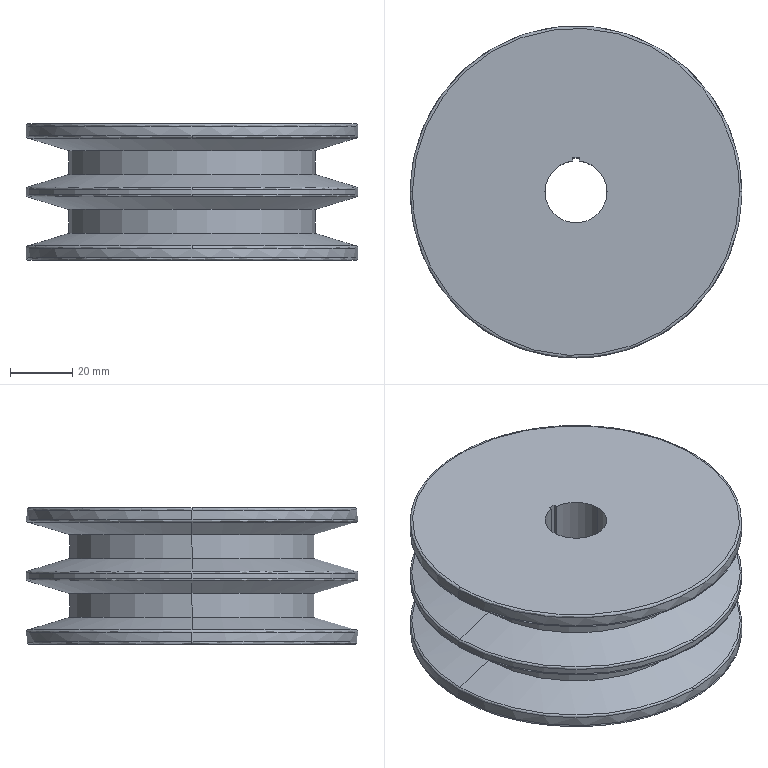Part | SolidWorks | features ICE 3, BaseBody 1 | 1 solid | 38 faces | box 107 x 107 x 44 mm | volume 283777 mm3 | cylinder 13 | spline 12 | cone 8 | plane 5 | commonest cylinder face diameters 107 x6 79.502 x4 20 x3
STEP:
#1=CARTESIAN_POINT('',(-52.969,0.,-4.592));
#2=VERTEX_POINT('',#1);
#3=CARTESIAN_POINT('',(0.,-52.969,-4.592));
#4=VERTEX_POINT('',#3);
#5=CARTESIAN_POINT('',(0.,0.,-4.592));
#6=DIRECTION('',(0.,0.,1.));
#7=DIRECTION('',(0.,1.,0.));
#8=AXIS2_PLACEMENT_3D('',#5,#6,#7);
#9=CIRCLE('',#8,52.969);
#10=EDGE_CURVE('',#2,#4,#9,.T.);
#11=ORIENTED_EDGE('',*,*,#10,.T.);
#12=CARTESIAN_POINT('',(0.,-53.5,-3.875));
#13=VERTEX_POINT('',#12);
#14=CARTESIAN_POINT('',(0.,-52.75,-3.875));
#15=DIRECTION('',(-1.,0.,0.));
#16=DIRECTION('',(0.,-1.,0.));
#17=AXIS2_PLACEMENT_3D('',#14,#15,#16);
#18=CIRCLE('',#17,0.75);
#19=EDGE_CURVE('',#4,#13,#18,.T.);
#20=ORIENTED_EDGE('',*,*,#19,.T.);
#21=CARTESIAN_POINT('',(-53.5,0.,-3.875));
#22=VERTEX_POINT('',#21);
#23=CARTESIAN_POINT('',(0.,0.,-3.875));
#24=DIRECTION('',(0.,0.,1.));
#25=DIRECTION('',(1.,0.,0.));
#26=AXIS2_PLACEMENT_3D('',#23,#24,#25);
#27=CIRCLE('',#26,53.5);
#28=EDGE_CURVE('',#22,#13,#27,.T.);
#29=ORIENTED_EDGE('',*,*,#28,.F.);
#30=CARTESIAN_POINT('',(0.,53.5,-3.875));
#31=VERTEX_POINT('',#30);
#32=CARTESIAN_POINT('',(0.,0.,-3.875));
#33=DIRECTION('',(0.,0.,1.));
#34=DIRECTION('',(1.,0.,0.));
#35=AXIS2_PLACEMENT_3D('',#32,#33,#34);
#36=CIRCLE('',#35,53.5);
#37=EDGE_CURVE('',#31,#22,#36,.T.);
#38=ORIENTED_EDGE('',*,*,#37,.F.);
#39=CARTESIAN_POINT('',(0.,52.969,-4.592));
#40=VERTEX_POINT('',#39);
#41=CARTESIAN_POINT('',(0.,52.75,-3.875));
#42=DIRECTION('',(1.,0.,0.));
#43=DIRECTION('',(0.,1.,0.));
#44=AXIS2_PLACEMENT_3D('',#41,#42,#43);
#45=CIRCLE('',#44,0.75);
#46=EDGE_CURVE('',#40,#31,#45,.T.);
#47=ORIENTED_EDGE('',*,*,#46,.F.);
#48=CARTESIAN_POINT('',(0.,0.,-4.592));
#49=DIRECTION('',(0.,0.,1.));
#50=DIRECTION('',(0.,1.,0.));
#51=AXIS2_PLACEMENT_3D('',#48,#49,#50);
#52=CIRCLE('',#51,52.969);
#53=EDGE_CURVE('',#40,#2,#52,.T.);
#54=ORIENTED_EDGE('',*,*,#53,.T.);
#55=EDGE_LOOP('',(#11,#20,#29,#38,#47,#54));
#56=FACE_OUTER_BOUND('',#55,.T.);
#57=CARTESIAN_POINT('',(0.,-52.969,-4.592));
#58=CARTESIAN_POINT('',(-105.939,-52.969,-4.592));
#59=CARTESIAN_POINT('',(-105.939,52.969,-4.592));
#60=CARTESIAN_POINT('',(0.,52.969,-4.592));
#61=CARTESIAN_POINT('',(0.,-53.296,-4.492));
#62=CARTESIAN_POINT('',(-106.593,-53.296,-4.492));
#63=CARTESIAN_POINT('',(-106.593,53.296,-4.492));
#64=CARTESIAN_POINT('',(0.,53.296,-4.492));
#65=CARTESIAN_POINT('',(0.,-53.5,-4.217));
#66=CARTESIAN_POINT('',(-107.,-53.5,-4.217));
#67=CARTESIAN_POINT('',(-107.,53.5,-4.217));
#68=CARTESIAN_POINT('',(0.,53.5,-4.217));
#69=CARTESIAN_POINT('',(0.,-53.5,-3.875));
#70=CARTESIAN_POINT('',(-107.,-53.5,-3.875));
#71=CARTESIAN_POINT('',(-107.,53.5,-3.875));
#72=CARTESIAN_POINT('',(0.,53.5,-3.875));
#73=(BOUNDED_SURFACE()B_SPLINE_SURFACE(3,3,((#57,#58,#59,#60),(#61,#62,#63,#64),(#65,#66,#67,#68),(#69,#70,#71,#72)),.UNSPECIFIED.,.F.,.F.,.F.)B_SPLINE_SURFACE_WITH_KNOTS((4,4),(4,4),(0.,1.),(0.,1.),.UNSPECIFIED.)GEOMETRIC_REPRESENTATION_ITEM()RATIONAL_B_SPLINE_SURFACE(((1.,0.3333,0.3333,1.),(0.8692,0.2897,0.2897,0.8692),(0.8692,0.2897,0.2897,0.8692),(1.,0.3333,0.3333,1.)))REPRESENTATION_ITEM('')SURFACE());
#74=ADVANCED_FACE('',(#56),#73,.T.);
#75=CARTESIAN_POINT('',(-53.5,0.,-0.75));
#76=VERTEX_POINT('',#75);
#77=CARTESIAN_POINT('',(53.5,0.,-0.75));
#78=VERTEX_POINT('',#77);
#79=CARTESIAN_POINT('',(0.,0.,-0.75));
#80=DIRECTION('',(0.,0.,1.));
#81=DIRECTION('',(-1.,0.,0.));
#82=AXIS2_PLACEMENT_3D('',#79,#80,#81);
#83=CIRCLE('',#82,53.5);
#84=EDGE_CURVE('',#76,#78,#83,.T.);
#85=ORIENTED_EDGE('',*,*,#84,.T.);
#86=CARTESIAN_POINT('',(52.75,0.,0.));
#87=VERTEX_POINT('',#86);
#88=CARTESIAN_POINT('',(52.75,0.,-0.75));
#89=DIRECTION('',(0.,-1.,0.));
#90=DIRECTION('',(1.,0.,0.));
#91=AXIS2_PLACEMENT_3D('',#88,#89,#90);
#92=CIRCLE('',#91,0.75);
#93=EDGE_CURVE('',#78,#87,#92,.T.);
#94=ORIENTED_EDGE('',*,*,#93,.T.);
#95=CARTESIAN_POINT('',(-52.75,0.,0.));
#96=VERTEX_POINT('',#95);
#97=CARTESIAN_POINT('',(52.75,0.,0.));
#98=CARTESIAN_POINT('',(52.75,-105.5,0.));
#99=CARTESIAN_POINT('',(-52.75,-105.5,0.));
#100=CARTESIAN_POINT('',(-52.75,0.,0.));
#101=(BOUNDED_CURVE()B_SPLINE_CURVE(3,(#97,#98,#99,#100),.UNSPECIFIED.,.F.,.F.)B_SPLINE_CURVE_WITH_KNOTS((4,4),(0.,1.),.UNSPECIFIED.)CURVE()GEOMETRIC_REPRESENTATION_ITEM()RATIONAL_B_SPLINE_CURVE((1.,0.3333,0.3333,1.))REPRESENTATION_ITEM(''));
#102=EDGE_CURVE('',#87,#96,#101,.T.);
#103=ORIENTED_EDGE('',*,*,#102,.T.);
#104=CARTESIAN_POINT('',(-52.75,0.,-0.75));
#105=DIRECTION('',(0.,1.,0.));
#106=DIRECTION('',(-1.,0.,0.));
#107=AXIS2_PLACEMENT_3D('',#104,#105,#106);
#108=CIRCLE('',#107,0.75);
#109=EDGE_CURVE('',#76,#96,#108,.T.);
#110=ORIENTED_EDGE('',*,*,#109,.F.);
#111=EDGE_LOOP('',(#85,#94,#103,#110));
#112=FACE_OUTER_BOUND('',#111,.T.);
#113=CARTESIAN_POINT('',(53.5,0.,-0.75));
#114=CARTESIAN_POINT('',(53.5,-107.,-0.75));
#115=CARTESIAN_POINT('',(-53.5,-107.,-0.75));
#116=CARTESIAN_POINT('',(-53.5,0.,-0.75));
#117=CARTESIAN_POINT('',(53.5,0.,-0.3107));
#118=CARTESIAN_POINT('',(53.5,-107.,-0.3107));
#119=CARTESIAN_POINT('',(-53.5,-107.,-0.3107));
#120=CARTESIAN_POINT('',(-53.5,0.,-0.3107));
#121=CARTESIAN_POINT('',(53.189,0.,0.));
#122=CARTESIAN_POINT('',(53.189,-106.379,0.));
#123=CARTESIAN_POINT('',(-53.189,-106.379,0.));
#124=CARTESIAN_POINT('',(-53.189,0.,0.));
#125=CARTESIAN_POINT('',(52.75,0.,0.));
#126=CARTESIAN_POINT('',(52.75,-105.5,0.));
#127=CARTESIAN_POINT('',(-52.75,-105.5,0.));
#128=CARTESIAN_POINT('',(-52.75,0.,0.));
#129=(BOUNDED_SURFACE()B_SPLINE_SURFACE(3,3,((#113,#114,#115,#116),(#117,#118,#119,#120),(#121,#122,#123,#124),(#125,#126,#127,#128)),.UNSPECIFIED.,.F.,.F.,.T.)B_SPLINE_SURFACE_WITH_KNOTS((4,4),(4,4),(0.,1.),(0.,1.),.UNSPECIFIED.)GEOMETRIC_REPRESENTATION_ITEM()RATIONAL_B_SPLINE_SURFACE(((1.,0.3333,0.3333,1.),(0.8047,0.2682,0.2682,0.8047),(0.8047,0.2682,0.2682,0.8047),(1.,0.3333,0.3333,1.)))REPRESENTATION_ITEM('')SURFACE());
#130=ADVANCED_FACE('',(#112),#129,.T.);
#131=CARTESIAN_POINT('',(-53.5,0.,-21.125));
#132=VERTEX_POINT('',#131);
#133=CARTESIAN_POINT('',(0.,-53.5,-21.125));
#134=VERTEX_POINT('',#133);
#135=CARTESIAN_POINT('',(0.,0.,-21.125));
#136=DIRECTION('',(0.,0.,1.));
#137=DIRECTION('',(0.,1.,0.));
#138=AXIS2_PLACEMENT_3D('',#135,#136,#137);
#139=CIRCLE('',#138,53.5);
#140=EDGE_CURVE('',#132,#134,#139,.T.);
#141=ORIENTED_EDGE('',*,*,#140,.T.);
#142=CARTESIAN_POINT('',(0.,-52.969,-20.408));
#143=VERTEX_POINT('',#142);
#144=CARTESIAN_POINT('',(0.,-52.75,-21.125));
#145=DIRECTION('',(-1.,0.,0.));
#146=DIRECTION('',(0.,-1.,0.));
#147=AXIS2_PLACEMENT_3D('',#144,#145,#146);
#148=CIRCLE('',#147,0.75);
#149=EDGE_CURVE('',#134,#143,#148,.T.);
#150=ORIENTED_EDGE('',*,*,#149,.T.);
#151=CARTESIAN_POINT('',(-52.969,0.,-20.408));
#152=VERTEX_POINT('',#151);
#153=CARTESIAN_POINT('',(0.,0.,-20.408));
#154=DIRECTION('',(0.,0.,1.));
#155=DIRECTION('',(0.,1.,0.));
#156=AXIS2_PLACEMENT_3D('',#153,#154,#155);
#157=CIRCLE('',#156,52.969);
#158=EDGE_CURVE('',#152,#143,#157,.T.);
#159=ORIENTED_EDGE('',*,*,#158,.F.);
#160=CARTESIAN_POINT('',(0.,52.969,-20.408));
#161=VERTEX_POINT('',#160);
#162=CARTESIAN_POINT('',(0.,0.,-20.408));
#163=DIRECTION('',(0.,0.,1.));
#164=DIRECTION('',(0.,1.,0.));
#165=AXIS2_PLACEMENT_3D('',#162,#163,#164);
#166=CIRCLE('',#165,52.969);
#167=EDGE_CURVE('',#161,#152,#166,.T.);
#168=ORIENTED_EDGE('',*,*,#167,.F.);
#169=CARTESIAN_POINT('',(0.,53.5,-21.125));
#170=VERTEX_POINT('',#169);
#171=CARTESIAN_POINT('',(0.,52.75,-21.125));
#172=DIRECTION('',(1.,0.,0.));
#173=DIRECTION('',(0.,1.,0.));
#174=AXIS2_PLACEMENT_3D('',#171,#172,#173);
#175=CIRCLE('',#174,0.75);
#176=EDGE_CURVE('',#170,#161,#175,.T.);
#177=ORIENTED_EDGE('',*,*,#176,.F.);
#178=CARTESIAN_POINT('',(0.,0.,-21.125));
#179=DIRECTION('',(0.,0.,1.));
#180=DIRECTION('',(0.,1.,0.));
#181=AXIS2_PLACEMENT_3D('',#178,#179,#180);
#182=CIRCLE('',#181,53.5);
#183=EDGE_CURVE('',#170,#132,#182,.T.);
#184=ORIENTED_EDGE('',*,*,#183,.T.);
#185=EDGE_LOOP('',(#141,#150,#159,#168,#177,#184));
#186=FACE_OUTER_BOUND('',#185,.T.);
#187=CARTESIAN_POINT('',(0.,-53.5,-21.125));
#188=CARTESIAN_POINT('',(-107.,-53.5,-21.125));
#189=CARTESIAN_POINT('',(-107.,53.5,-21.125));
#190=CARTESIAN_POINT('',(0.,53.5,-21.125));
#191=CARTESIAN_POINT('',(0.,-53.5,-20.783));
#192=CARTESIAN_POINT('',(-107.,-53.5,-20.783));
#193=CARTESIAN_POINT('',(-107.,53.5,-20.783));
#194=CARTESIAN_POINT('',(0.,53.5,-20.783));
#195=CARTESIAN_POINT('',(0.,-53.296,-20.508));
#196=CARTESIAN_POINT('',(-106.593,-53.296,-20.508));
#197=CARTESIAN_POINT('',(-106.593,53.296,-20.508));
#198=CARTESIAN_POINT('',(0.,53.296,-20.508));
#199=CARTESIAN_POINT('',(0.,-52.969,-20.408));
#200=CARTESIAN_POINT('',(-105.939,-52.969,-20.408));
#201=CARTESIAN_POINT('',(-105.939,52.969,-20.408));
#202=CARTESIAN_POINT('',(0.,52.969,-20.408));
#203=(BOUNDED_SURFACE()B_SPLINE_SURFACE(3,3,((#187,#188,#189,#190),(#191,#192,#193,#194),(#195,#196,#197,#198),(#199,#200,#201,#202)),.UNSPECIFIED.,.F.,.F.,.T.)B_SPLINE_SURFACE_WITH_KNOTS((4,4),(4,4),(0.,1.),(0.,1.),.UNSPECIFIED.)GEOMETRIC_REPRESENTATION_ITEM()RATIONAL_B_SPLINE_SURFACE(((1.,0.3333,0.3333,1.),(0.8692,0.2897,0.2897,0.8692),(0.8692,0.2897,0.2897,0.8692),(1.,0.3333,0.3333,1.)))REPRESENTATION_ITEM('')SURFACE());
#204=ADVANCED_FACE('',(#186),#203,.T.);
#205=CARTESIAN_POINT('',(-52.969,0.,-23.592));
#206=VERTEX_POINT('',#205);
#207=CARTESIAN_POINT('',(0.,-52.969,-23.592));
#208=VERTEX_POINT('',#207);
#209=CARTESIAN_POINT('',(0.,0.,-23.592));
#210=DIRECTION('',(0.,0.,1.));
#211=DIRECTION('',(0.,1.,0.));
#212=AXIS2_PLACEMENT_3D('',#209,#210,#211);
#213=CIRCLE('',#212,52.969);
#214=EDGE_CURVE('',#206,#208,#213,.T.);
#215=ORIENTED_EDGE('',*,*,#214,.T.);
#216=CARTESIAN_POINT('',(0.,-53.5,-22.875));
#217=VERTEX_POINT('',#216);
#218=CARTESIAN_POINT('',(0.,-52.75,-22.875));
#219=DIRECTION('',(-1.,0.,0.));
#220=DIRECTION('',(0.,-1.,0.));
#221=AXIS2_PLACEMENT_3D('',#218,#219,#220);
#222=CIRCLE('',#221,0.75);
#223=EDGE_CURVE('',#208,#217,#222,.T.);
#224=ORIENTED_EDGE('',*,*,#223,.T.);
#225=CARTESIAN_POINT('',(-53.5,0.,-22.875));
#226=VERTEX_POINT('',#225);
#227=CARTESIAN_POINT('',(0.,0.,-22.875));
#228=DIRECTION('',(0.,0.,1.));
#229=DIRECTION('',(1.,0.,0.));
#230=AXIS2_PLACEMENT_3D('',#227,#228,#229);
#231=CIRCLE('',#230,53.5);
#232=EDGE_CURVE('',#226,#217,#231,.T.);
#233=ORIENTED_EDGE('',*,*,#232,.F.);
#234=CARTESIAN_POINT('',(0.,53.5,-22.875));
#235=VERTEX_POINT('',#234);
#236=CARTESIAN_POINT('',(0.,0.,-22.875));
#237=DIRECTION('',(0.,0.,1.));
#238=DIRECTION('',(1.,0.,0.));
#239=AXIS2_PLACEMENT_3D('',#236,#237,#238);
#240=CIRCLE('',#239,53.5);
#241=EDGE_CURVE('',#235,#226,#240,.T.);
#242=ORIENTED_EDGE('',*,*,#241,.F.);
#243=CARTESIAN_POINT('',(0.,52.969,-23.592));
#244=VERTEX_POINT('',#243);
#245=CARTESIAN_POINT('',(0.,52.75,-22.875));
#246=DIRECTION('',(1.,0.,0.));
#247=DIRECTION('',(0.,1.,0.));
#248=AXIS2_PLACEMENT_3D('',#245,#246,#247);
#249=CIRCLE('',#248,0.75);
#250=EDGE_CURVE('',#244,#235,#249,.T.);
#251=ORIENTED_EDGE('',*,*,#250,.F.);
#252=CARTESIAN_POINT('',(0.,0.,-23.592));
#253=DIRECTION('',(0.,0.,1.));
#254=DIRECTION('',(0.,1.,0.));
#255=AXIS2_PLACEMENT_3D('',#252,#253,#254);
#256=CIRCLE('',#255,52.969);
#257=EDGE_CURVE('',#244,#206,#256,.T.);
#258=ORIENTED_EDGE('',*,*,#257,.T.);
#259=EDGE_LOOP('',(#215,#224,#233,#242,#251,#258));
#260=FACE_OUTER_BOUND('',#259,.T.);
#261=CARTESIAN_POINT('',(0.,-52.969,-23.592));
#262=CARTESIAN_POINT('',(-105.939,-52.969,-23.592));
#263=CARTESIAN_POINT('',(-105.939,52.969,-23.592));
#264=CARTESIAN_POINT('',(0.,52.969,-23.592));
#265=CARTESIAN_POINT('',(0.,-53.296,-23.492));
#266=CARTESIAN_POINT('',(-106.593,-53.296,-23.492));
#267=CARTESIAN_POINT('',(-106.593,53.296,-23.492));
#268=CARTESIAN_POINT('',(0.,53.296,-23.492));
#269=CARTESIAN_POINT('',(0.,-53.5,-23.217));
#270=CARTESIAN_POINT('',(-107.,-53.5,-23.217));
#271=CARTESIAN_POINT('',(-107.,53.5,-23.217));
#272=CARTESIAN_POINT('',(0.,53.5,-23.217));
#273=CARTESIAN_POINT('',(0.,-53.5,-22.875));
#274=CARTESIAN_POINT('',(-107.,-53.5,-22.875));
#275=CARTESIAN_POINT('',(-107.,53.5,-22.875));
#276=CARTESIAN_POINT('',(0.,53.5,-22.875));
#277=(BOUNDED_SURFACE()B_SPLINE_SURFACE(3,3,((#261,#262,#263,#264),(#265,#266,#267,#268),(#269,#270,#271,#272),(#273,#274,#275,#276)),.UNSPECIFIED.,.F.,.F.,.F.)B_SPLINE_SURFACE_WITH_KNOTS((4,4),(4,4),(0.,1.),(0.,1.),.UNSPECIFIED.)GEOMETRIC_REPRESENTATION_ITEM()RATIONAL_B_SPLINE_SURFACE(((1.,0.3333,0.3333,1.),(0.8692,0.2897,0.2897,0.8692),(0.8692,0.2897,0.2897,0.8692),(1.,0.3333,0.3333,1.)))REPRESENTATION_ITEM('')SURFACE());
#278=ADVANCED_FACE('',(#260),#277,.T.);
#279=CARTESIAN_POINT('',(53.5,0.,-43.25));
#280=VERTEX_POINT('',#279);
#281=CARTESIAN_POINT('',(-53.5,0.,-43.25));
#282=VERTEX_POINT('',#281);
#283=CARTESIAN_POINT('',(0.,0.,-43.25));
#284=DIRECTION('',(0.,0.,-1.));
#285=DIRECTION('',(1.,0.,0.));
#286=AXIS2_PLACEMENT_3D('',#283,#284,#285);
#287=CIRCLE('',#286,53.5);
#288=EDGE_CURVE('',#280,#282,#287,.T.);
#289=ORIENTED_EDGE('',*,*,#288,.T.);
#290=CARTESIAN_POINT('',(-52.75,0.,-44.));
#291=VERTEX_POINT('',#290);
#292=CARTESIAN_POINT('',(-52.75,0.,-43.25));
#293=DIRECTION('',(0.,-1.,0.));
#294=DIRECTION('',(-1.,0.,0.));
#295=AXIS2_PLACEMENT_3D('',#292,#293,#294);
#296=CIRCLE('',#295,0.75);
#297=EDGE_CURVE('',#282,#291,#296,.T.);
#298=ORIENTED_EDGE('',*,*,#297,.T.);
#299=CARTESIAN_POINT('',(52.75,0.,-44.));
#300=VERTEX_POINT('',#299);
#301=CARTESIAN_POINT('',(-52.75,0.,-44.));
#302=CARTESIAN_POINT('',(-52.75,-105.5,-44.));
#303=CARTESIAN_POINT('',(52.75,-105.5,-44.));
#304=CARTESIAN_POINT('',(52.75,0.,-44.));
#305=(BOUNDED_CURVE()B_SPLINE_CURVE(3,(#301,#302,#303,#304),.UNSPECIFIED.,.F.,.F.)B_SPLINE_CURVE_WITH_KNOTS((4,4),(0.,1.),.UNSPECIFIED.)CURVE()GEOMETRIC_REPRESENTATION_ITEM()RATIONAL_B_SPLINE_CURVE((1.,0.3333,0.3333,1.))REPRESENTATION_ITEM(''));
#306=EDGE_CURVE('',#291,#300,#305,.T.);
#307=ORIENTED_EDGE('',*,*,#306,.T.);
#308=CARTESIAN_POINT('',(52.75,0.,-43.25));
#309=DIRECTION('',(0.,1.,0.));
#310=DIRECTION('',(1.,0.,0.));
#311=AXIS2_PLACEMENT_3D('',#308,#309,#310);
#312=CIRCLE('',#311,0.75);
#313=EDGE_CURVE('',#280,#300,#312,.T.);
#314=ORIENTED_EDGE('',*,*,#313,.F.);
#315=EDGE_LOOP('',(#289,#298,#307,#314));
#316=FACE_OUTER_BOUND('',#315,.T.);
#317=CARTESIAN_POINT('',(-53.5,0.,-43.25));
#318=CARTESIAN_POINT('',(-53.5,-107.,-43.25));
#319=CARTESIAN_POINT('',(53.5,-107.,-43.25));
#320=CARTESIAN_POINT('',(53.5,0.,-43.25));
#321=CARTESIAN_POINT('',(-53.5,0.,-43.689));
#322=CARTESIAN_POINT('',(-53.5,-107.,-43.689));
#323=CARTESIAN_POINT('',(53.5,-107.,-43.689));
#324=CARTESIAN_POINT('',(53.5,0.,-43.689));
#325=CARTESIAN_POINT('',(-53.189,0.,-44.));
#326=CARTESIAN_POINT('',(-53.189,-106.379,-44.));
#327=CARTESIAN_POINT('',(53.189,-106.379,-44.));
#328=CARTESIAN_POINT('',(53.189,0.,-44.));
#329=CARTESIAN_POINT('',(-52.75,0.,-44.));
#330=CARTESIAN_POINT('',(-52.75,-105.5,-44.));
#331=CARTESIAN_POINT('',(52.75,-105.5,-44.));
#332=CARTESIAN_POINT('',(52.75,0.,-44.));
#333=(BOUNDED_SURFACE()B_SPLINE_SURFACE(3,3,((#317,#318,#319,#320),(#321,#322,#323,#324),(#325,#326,#327,#328),(#329,#330,#331,#332)),.UNSPECIFIED.,.F.,.F.,.T.)B_SPLINE_SURFACE_WITH_KNOTS((4,4),(4,4),(0.,1.),(0.,1.),.UNSPECIFIED.)GEOMETRIC_REPRESENTATION_ITEM()RATIONAL_B_SPLINE_SURFACE(((1.,0.3333,0.3333,1.),(0.8047,0.2682,0.2682,0.8047),(0.8047,0.2682,0.2682,0.8047),(1.,0.3333,0.3333,1.)))REPRESENTATION_ITEM('')SURFACE());
#334=ADVANCED_FACE('',(#316),#333,.T.);
#335=CARTESIAN_POINT('',(0.,-53.5,-40.125));
#336=VERTEX_POINT('',#335);
#337=CARTESIAN_POINT('',(-53.5,0.,-40.125));
#338=VERTEX_POINT('',#337);
#339=CARTESIAN_POINT('',(0.,0.,-40.125));
#340=DIRECTION('',(0.,0.,-1.));
#341=DIRECTION('',(1.,0.,0.));
#342=AXIS2_PLACEMENT_3D('',#339,#340,#341);
#343=CIRCLE('',#342,53.5);
#344=EDGE_CURVE('',#336,#338,#343,.T.);
#345=ORIENTED_EDGE('',*,*,#344,.F.);
#346=CARTESIAN_POINT('',(0.,-52.969,-39.408));
#347=VERTEX_POINT('',#346);
#348=CARTESIAN_POINT('',(0.,-52.75,-40.125));
#349=DIRECTION('',(-1.,0.,0.));
#350=DIRECTION('',(0.,-1.,0.));
#351=AXIS2_PLACEMENT_3D('',#348,#349,#350);
#352=CIRCLE('',#351,0.75);
#353=EDGE_CURVE('',#336,#347,#352,.T.);
#354=ORIENTED_EDGE('',*,*,#353,.T.);
#355=CARTESIAN_POINT('',(-52.969,0.,-39.408));
#356=VERTEX_POINT('',#355);
#357=CARTESIAN_POINT('',(0.,0.,-39.408));
#358=DIRECTION('',(0.,0.,-1.));
#359=DIRECTION('',(0.,1.,0.));
#360=AXIS2_PLACEMENT_3D('',#357,#358,#359);
#361=CIRCLE('',#360,52.969);
#362=EDGE_CURVE('',#347,#356,#361,.T.);
#363=ORIENTED_EDGE('',*,*,#362,.T.);
#364=CARTESIAN_POINT('',(0.,52.969,-39.408));
#365=VERTEX_POINT('',#364);
#366=CARTESIAN_POINT('',(0.,0.,-39.408));
#367=DIRECTION('',(0.,0.,-1.));
#368=DIRECTION('',(0.,1.,0.));
#369=AXIS2_PLACEMENT_3D('',#366,#367,#368);
#370=CIRCLE('',#369,52.969);
#371=EDGE_CURVE('',#356,#365,#370,.T.);
#372=ORIENTED_EDGE('',*,*,#371,.T.);
#373=CARTESIAN_POINT('',(0.,53.5,-40.125));
#374=VERTEX_POINT('',#373);
#375=CARTESIAN_POINT('',(0.,52.75,-40.125));
#376=DIRECTION('',(1.,0.,0.));
#377=DIRECTION('',(0.,1.,0.));
#378=AXIS2_PLACEMENT_3D('',#375,#376,#377);
#379=CIRCLE('',#378,0.75);
#380=EDGE_CURVE('',#374,#365,#379,.T.);
#381=ORIENTED_EDGE('',*,*,#380,.F.);
#382=CARTESIAN_POINT('',(0.,0.,-40.125));
#383=DIRECTION('',(0.,0.,-1.));
#384=DIRECTION('',(1.,0.,0.));
#385=AXIS2_PLACEMENT_3D('',#382,#383,#384);
#386=CIRCLE('',#385,53.5);
#387=EDGE_CURVE('',#338,#374,#386,.T.);
#388=ORIENTED_EDGE('',*,*,#387,.F.);
#389=EDGE_LOOP('',(#345,#354,#363,#372,#381,#388));
#390=FACE_OUTER_BOUND('',#389,.T.);
#391=CARTESIAN_POINT('',(0.,-53.5,-40.125));
#392=CARTESIAN_POINT('',(-107.,-53.5,-40.125));
#393=CARTESIAN_POINT('',(-107.,53.5,-40.125));
#394=CARTESIAN_POINT('',(0.,53.5,-40.125));
#395=CARTESIAN_POINT('',(0.,-53.5,-39.783));
#396=CARTESIAN_POINT('',(-107.,-53.5,-39.783));
#397=CARTESIAN_POINT('',(-107.,53.5,-39.783));
#398=CARTESIAN_POINT('',(0.,53.5,-39.783));
#399=CARTESIAN_POINT('',(0.,-53.296,-39.508));
#400=CARTESIAN_POINT('',(-106.593,-53.296,-39.508));
#401=CARTESIAN_POINT('',(-106.593,53.296,-39.508));
#402=CARTESIAN_POINT('',(0.,53.296,-39.508));
#403=CARTESIAN_POINT('',(0.,-52.969,-39.408));
#404=CARTESIAN_POINT('',(-105.939,-52.969,-39.408));
#405=CARTESIAN_POINT('',(-105.939,52.969,-39.408));
#406=CARTESIAN_POINT('',(0.,52.969,-39.408));
#407=(BOUNDED_SURFACE()B_SPLINE_SURFACE(3,3,((#391,#392,#393,#394),(#395,#396,#397,#398),(#399,#400,#401,#402),(#403,#404,#405,#406)),.UNSPECIFIED.,.F.,.F.,.F.)B_SPLINE_SURFACE_WITH_KNOTS((4,4),(4,4),(0.,1.),(0.,1.),.UNSPECIFIED.)GEOMETRIC_REPRESENTATION_ITEM()RATIONAL_B_SPLINE_SURFACE(((1.,0.3333,0.3333,1.),(0.8692,0.2897,0.2897,0.8692),(0.8692,0.2897,0.2897,0.8692),(1.,0.3333,0.3333,1.)))REPRESENTATION_ITEM('')SURFACE());
#408=ADVANCED_FACE('',(#390),#407,.T.);
#409=CARTESIAN_POINT('',(-10.,0.,-44.));
#410=VERTEX_POINT('',#409);
#411=CARTESIAN_POINT('',(10.,0.,-44.));
#412=VERTEX_POINT('',#411);
#413=CARTESIAN_POINT('',(0.,0.,-44.));
#414=DIRECTION('',(0.,0.,1.));
#415=DIRECTION('',(1.,0.,0.));
#416=AXIS2_PLACEMENT_3D('',#413,#414,#415);
#417=CIRCLE('',#416,10.);
#418=EDGE_CURVE('',#410,#412,#417,.T.);
#419=ORIENTED_EDGE('',*,*,#418,.F.);
#420=CARTESIAN_POINT('',(-10.,0.,0.));
#421=VERTEX_POINT('',#420);
#422=CARTESIAN_POINT('',(-10.,0.,-44.004));
#423=DIRECTION('',(0.,0.,1.));
#424=VECTOR('',#423,1000.);
#425=LINE('',#422,#424);
#426=EDGE_CURVE('',#410,#421,#425,.T.);
#427=ORIENTED_EDGE('',*,*,#426,.T.);
#428=CARTESIAN_POINT('',(10.,0.,0.));
#429=VERTEX_POINT('',#428);
#430=CARTESIAN_POINT('',(0.,0.,0.));
#431=DIRECTION('',(0.,0.,1.));
#432=DIRECTION('',(1.,0.,0.));
#433=AXIS2_PLACEMENT_3D('',#430,#431,#432);
#434=CIRCLE('',#433,10.);
#435=EDGE_CURVE('',#421,#429,#434,.T.);
#436=ORIENTED_EDGE('',*,*,#435,.T.);
#437=CARTESIAN_POINT('',(10.,0.,-44.004));
#438=DIRECTION('',(0.,0.,1.));
#439=VECTOR('',#438,1000.);
#440=LINE('',#437,#439);
#441=EDGE_CURVE('',#412,#429,#440,.T.);
#442=ORIENTED_EDGE('',*,*,#441,.F.);
#443=EDGE_LOOP('',(#419,#427,#436,#442));
#444=FACE_OUTER_BOUND('',#443,.T.);
#445=CARTESIAN_POINT('',(0.,0.,-44.004));
#446=DIRECTION('',(0.,0.,1.));
#447=DIRECTION('',(1.,0.,0.));
#448=AXIS2_PLACEMENT_3D('',#445,#446,#447);
#449=CYLINDRICAL_SURFACE('',#448,10.);
#450=ADVANCED_FACE('',(#444),#449,.F.);
#451=CARTESIAN_POINT('',(1.,9.95,-44.));
#452=VERTEX_POINT('',#451);
#453=CARTESIAN_POINT('',(0.,0.,-44.));
#454=DIRECTION('',(0.,0.,1.));
#455=DIRECTION('',(1.,0.,0.));
#456=AXIS2_PLACEMENT_3D('',#453,#454,#455);
#457=CIRCLE('',#456,10.);
#458=EDGE_CURVE('',#412,#452,#457,.T.);
#459=ORIENTED_EDGE('',*,*,#458,.F.);
#460=ORIENTED_EDGE('',*,*,#441,.T.);
#461=CARTESIAN_POINT('',(1.,9.95,0.));
#462=VERTEX_POINT('',#461);
#463=CARTESIAN_POINT('',(0.,0.,0.));
#464=DIRECTION('',(0.,0.,1.));
#465=DIRECTION('',(1.,0.,0.));
#466=AXIS2_PLACEMENT_3D('',#463,#464,#465);
#467=CIRCLE('',#466,10.);
#468=EDGE_CURVE('',#429,#462,#467,.T.);
#469=ORIENTED_EDGE('',*,*,#468,.T.);
#470=CARTESIAN_POINT('',(1.,9.95,-44.004));
#471=DIRECTION('',(0.,0.,-1.));
#472=VECTOR('',#471,1000.);
#473=LINE('',#470,#472);
#474=EDGE_CURVE('',#462,#452,#473,.T.);
#475=ORIENTED_EDGE('',*,*,#474,.T.);
#476=EDGE_LOOP('',(#459,#460,#469,#475));
#477=FACE_OUTER_BOUND('',#476,.T.);
#478=CARTESIAN_POINT('',(0.,0.,-44.004));
#479=DIRECTION('',(0.,0.,1.));
#480=DIRECTION('',(1.,0.,0.));
#481=AXIS2_PLACEMENT_3D('',#478,#479,#480);
#482=CYLINDRICAL_SURFACE('',#481,10.);
#483=ADVANCED_FACE('',(#477),#482,.F.);
#484=CARTESIAN_POINT('',(-39.751,0.,-8.633));
#485=VERTEX_POINT('',#484);
#486=CARTESIAN_POINT('',(39.751,0.,-8.633));
#487=VERTEX_POINT('',#486);
#488=CARTESIAN_POINT('',(0.,0.,-8.633));
#489=DIRECTION('',(0.,0.,-1.));
#490=DIRECTION('',(1.,0.,0.));
#491=AXIS2_PLACEMENT_3D('',#488,#489,#490);
#492=CIRCLE('',#491,39.751);
#493=EDGE_CURVE('',#485,#487,#492,.T.);
#494=ORIENTED_EDGE('',*,*,#493,.F.);
#495=CARTESIAN_POINT('',(-52.969,0.,-4.592));
#496=DIRECTION('',(-0.9563,0.,0.2924));
#497=VECTOR('',#496,1000.);
#498=LINE('',#495,#497);
#499=EDGE_CURVE('',#485,#2,#498,.T.);
#500=ORIENTED_EDGE('',*,*,#499,.T.);
#501=ORIENTED_EDGE('',*,*,#53,.F.);
#502=CARTESIAN_POINT('',(52.969,0.,-4.592));
#503=VERTEX_POINT('',#502);
#504=CARTESIAN_POINT('',(0.,0.,-4.592));
#505=DIRECTION('',(0.,0.,1.));
#506=DIRECTION('',(0.,1.,0.));
#507=AXIS2_PLACEMENT_3D('',#504,#505,#506);
#508=CIRCLE('',#507,52.969);
#509=EDGE_CURVE('',#503,#40,#508,.T.);
#510=ORIENTED_EDGE('',*,*,#509,.F.);
#511=CARTESIAN_POINT('',(52.969,0.,-4.592));
#512=DIRECTION('',(0.9563,0.,0.2924));
#513=VECTOR('',#512,1000.);
#514=LINE('',#511,#513);
#515=EDGE_CURVE('',#487,#503,#514,.T.);
#516=ORIENTED_EDGE('',*,*,#515,.F.);
#517=EDGE_LOOP('',(#494,#500,#501,#510,#516));
#518=FACE_OUTER_BOUND('',#517,.T.);
#519=CARTESIAN_POINT('',(0.,0.,-4.592));
#520=DIRECTION('',(0.,0.,1.));
#521=DIRECTION('',(1.,0.,0.));
#522=AXIS2_PLACEMENT_3D('',#519,#520,#521);
#523=CONICAL_SURFACE('',#522,52.969,1.274);
#524=ADVANCED_FACE('',(#518),#523,.T.);
#525=CARTESIAN_POINT('',(53.5,0.,-3.875));
#526=VERTEX_POINT('',#525);
#527=CARTESIAN_POINT('',(0.,0.,-3.875));
#528=DIRECTION('',(0.,0.,1.));
#529=DIRECTION('',(1.,0.,0.));
#530=AXIS2_PLACEMENT_3D('',#527,#528,#529);
#531=CIRCLE('',#530,53.5);
#532=EDGE_CURVE('',#526,#31,#531,.T.);
#533=ORIENTED_EDGE('',*,*,#532,.T.);
#534=ORIENTED_EDGE('',*,*,#37,.T.);
#535=CARTESIAN_POINT('',(-53.5,0.,0.));
#536=DIRECTION('',(0.,0.,1.));
#537=VECTOR('',#536,1000.);
#538=LINE('',#535,#537);
#539=EDGE_CURVE('',#22,#76,#538,.T.);
#540=ORIENTED_EDGE('',*,*,#539,.T.);
#541=CARTESIAN_POINT('',(0.,0.,-0.75));
#542=DIRECTION('',(0.,0.,1.));
#543=DIRECTION('',(-1.,0.,0.));
#544=AXIS2_PLACEMENT_3D('',#541,#542,#543);
#545=CIRCLE('',#544,53.5);
#546=EDGE_CURVE('',#78,#76,#545,.T.);
#547=ORIENTED_EDGE('',*,*,#546,.F.);
#548=CARTESIAN_POINT('',(53.5,0.,0.));
#549=DIRECTION('',(0.,0.,1.));
#550=VECTOR('',#549,1000.);
#551=LINE('',#548,#550);
#552=EDGE_CURVE('',#526,#78,#551,.T.);
#553=ORIENTED_EDGE('',*,*,#552,.F.);
#554=EDGE_LOOP('',(#533,#534,#540,#547,#553));
#555=FACE_OUTER_BOUND('',#554,.T.);
#556=CARTESIAN_POINT('',(0.,0.,0.));
#557=DIRECTION('',(0.,0.,1.));
#558=DIRECTION('',(1.,0.,0.));
#559=AXIS2_PLACEMENT_3D('',#556,#557,#558);
#560=CYLINDRICAL_SURFACE('',#559,53.5);
#561=ADVANCED_FACE('',(#555),#560,.T.);
#562=CARTESIAN_POINT('',(39.751,0.,-16.367));
#563=VERTEX_POINT('',#562);
#564=CARTESIAN_POINT('',(-39.751,0.,-16.367));
#565=VERTEX_POINT('',#564);
#566=CARTESIAN_POINT('',(0.,0.,-16.367));
#567=DIRECTION('',(0.,0.,1.));
#568=DIRECTION('',(-1.,0.,0.));
#569=AXIS2_PLACEMENT_3D('',#566,#567,#568);
#570=CIRCLE('',#569,39.751);
#571=EDGE_CURVE('',#563,#565,#570,.T.);
#572=ORIENTED_EDGE('',*,*,#571,.T.);
#573=CARTESIAN_POINT('',(-39.751,0.,-156.433));
#574=DIRECTION('',(0.,0.,1.));
#575=VECTOR('',#574,1000.);
#576=LINE('',#573,#575);
#577=EDGE_CURVE('',#565,#485,#576,.T.);
#578=ORIENTED_EDGE('',*,*,#577,.T.);
#579=ORIENTED_EDGE('',*,*,#493,.T.);
#580=CARTESIAN_POINT('',(39.751,0.,-156.433));
#581=DIRECTION('',(0.,0.,1.));
#582=VECTOR('',#581,1000.);
#583=LINE('',#580,#582);
#584=EDGE_CURVE('',#563,#487,#583,.T.);
#585=ORIENTED_EDGE('',*,*,#584,.F.);
#586=EDGE_LOOP('',(#572,#578,#579,#585));
#587=FACE_OUTER_BOUND('',#586,.T.);
#588=CARTESIAN_POINT('',(0.,0.,-156.433));
#589=DIRECTION('',(0.,0.,1.));
#590=DIRECTION('',(1.,0.,0.));
#591=AXIS2_PLACEMENT_3D('',#588,#589,#590);
#592=CYLINDRICAL_SURFACE('',#591,39.751);
#593=ADVANCED_FACE('',(#587),#592,.T.);
#594=ORIENTED_EDGE('',*,*,#571,.F.);
#595=CARTESIAN_POINT('',(52.969,0.,-20.408));
#596=VERTEX_POINT('',#595);
#597=CARTESIAN_POINT('',(52.969,0.,-20.408));
#598=DIRECTION('',(0.9563,0.,-0.2924));
#599=VECTOR('',#598,1000.);
#600=LINE('',#597,#599);
#601=EDGE_CURVE('',#563,#596,#600,.T.);
#602=ORIENTED_EDGE('',*,*,#601,.T.);
#603=CARTESIAN_POINT('',(0.,0.,-20.408));
#604=DIRECTION('',(0.,0.,1.));
#605=DIRECTION('',(0.,1.,0.));
#606=AXIS2_PLACEMENT_3D('',#603,#604,#605);
#607=CIRCLE('',#606,52.969);
#608=EDGE_CURVE('',#596,#161,#607,.T.);
#609=ORIENTED_EDGE('',*,*,#608,.T.);
#610=ORIENTED_EDGE('',*,*,#167,.T.);
#611=CARTESIAN_POINT('',(-52.969,0.,-20.408));
#612=DIRECTION('',(-0.9563,0.,-0.2924));
#613=VECTOR('',#612,1000.);
#614=LINE('',#611,#613);
#615=EDGE_CURVE('',#565,#152,#614,.T.);
#616=ORIENTED_EDGE('',*,*,#615,.F.);
#617=EDGE_LOOP('',(#594,#602,#609,#610,#616));
#618=FACE_OUTER_BOUND('',#617,.T.);
#619=CARTESIAN_POINT('',(0.,0.,-20.408));
#620=DIRECTION('',(0.,0.,-1.));
#621=DIRECTION('',(-1.,0.,0.));
#622=AXIS2_PLACEMENT_3D('',#619,#620,#621);
#623=CONICAL_SURFACE('',#622,52.969,1.274);
#624=ADVANCED_FACE('',(#618),#623,.T.);
#625=CARTESIAN_POINT('',(53.5,0.,-22.875));
#626=VERTEX_POINT('',#625);
#627=CARTESIAN_POINT('',(0.,0.,-22.875));
#628=DIRECTION('',(0.,0.,1.));
#629=DIRECTION('',(1.,0.,0.));
#630=AXIS2_PLACEMENT_3D('',#627,#628,#629);
#631=CIRCLE('',#630,53.5);
#632=EDGE_CURVE('',#626,#235,#631,.T.);
#633=ORIENTED_EDGE('',*,*,#632,.T.);
#634=ORIENTED_EDGE('',*,*,#241,.T.);
#635=CARTESIAN_POINT('',(-53.5,0.,0.));
#636=DIRECTION('',(0.,0.,1.));
#637=VECTOR('',#636,1000.);
#638=LINE('',#635,#637);
#639=EDGE_CURVE('',#226,#132,#638,.T.);
#640=ORIENTED_EDGE('',*,*,#639,.T.);
#641=ORIENTED_EDGE('',*,*,#183,.F.);
#642=CARTESIAN_POINT('',(53.5,0.,-21.125));
#643=VERTEX_POINT('',#642);
#644=CARTESIAN_POINT('',(0.,0.,-21.125));
#645=DIRECTION('',(0.,0.,1.));
#646=DIRECTION('',(0.,1.,0.));
#647=AXIS2_PLACEMENT_3D('',#644,#645,#646);
#648=CIRCLE('',#647,53.5);
#649=EDGE_CURVE('',#643,#170,#648,.T.);
#650=ORIENTED_EDGE('',*,*,#649,.F.);
#651=CARTESIAN_POINT('',(53.5,0.,0.));
#652=DIRECTION('',(0.,0.,1.));
#653=VECTOR('',#652,1000.);
#654=LINE('',#651,#653);
#655=EDGE_CURVE('',#626,#643,#654,.T.);
#656=ORIENTED_EDGE('',*,*,#655,.F.);
#657=EDGE_LOOP('',(#633,#634,#640,#641,#650,#656));
#658=FACE_OUTER_BOUND('',#657,.T.);
#659=CARTESIAN_POINT('',(0.,0.,0.));
#660=DIRECTION('',(0.,0.,1.));
#661=DIRECTION('',(1.,0.,0.));
#662=AXIS2_PLACEMENT_3D('',#659,#660,#661);
#663=CYLINDRICAL_SURFACE('',#662,53.5);
#664=ADVANCED_FACE('',(#658),#663,.T.);
#665=CARTESIAN_POINT('',(-39.751,0.,-27.633));
#666=VERTEX_POINT('',#665);
#667=CARTESIAN_POINT('',(39.751,0.,-27.633));
#668=VERTEX_POINT('',#667);
#669=CARTESIAN_POINT('',(0.,0.,-27.633));
#670=DIRECTION('',(0.,0.,-1.));
#671=DIRECTION('',(1.,0.,0.));
#672=AXIS2_PLACEMENT_3D('',#669,#670,#671);
#673=CIRCLE('',#672,39.751);
#674=EDGE_CURVE('',#666,#668,#673,.T.);
#675=ORIENTED_EDGE('',*,*,#674,.F.);
#676=CARTESIAN_POINT('',(-52.969,0.,-23.592));
#677=DIRECTION('',(-0.9563,0.,0.2924));
#678=VECTOR('',#677,1000.);
#679=LINE('',#676,#678);
#680=EDGE_CURVE('',#666,#206,#679,.T.);
#681=ORIENTED_EDGE('',*,*,#680,.T.);
#682=ORIENTED_EDGE('',*,*,#257,.F.);
#683=CARTESIAN_POINT('',(52.969,0.,-23.592));
#684=VERTEX_POINT('',#683);
#685=CARTESIAN_POINT('',(0.,0.,-23.592));
#686=DIRECTION('',(0.,0.,1.));
#687=DIRECTION('',(0.,1.,0.));
#688=AXIS2_PLACEMENT_3D('',#685,#686,#687);
#689=CIRCLE('',#688,52.969);
#690=EDGE_CURVE('',#684,#244,#689,.T.);
#691=ORIENTED_EDGE('',*,*,#690,.F.);
#692=CARTESIAN_POINT('',(52.969,0.,-23.592));
#693=DIRECTION('',(0.9563,0.,0.2924));
#694=VECTOR('',#693,1000.);
#695=LINE('',#692,#694);
#696=EDGE_CURVE('',#668,#684,#695,.T.);
#697=ORIENTED_EDGE('',*,*,#696,.F.);
#698=EDGE_LOOP('',(#675,#681,#682,#691,#697));
#699=FACE_OUTER_BOUND('',#698,.T.);
#700=CARTESIAN_POINT('',(0.,0.,-23.592));
#701=DIRECTION('',(0.,0.,1.));
#702=DIRECTION('',(1.,0.,0.));
#703=AXIS2_PLACEMENT_3D('',#700,#701,#702);
#704=CONICAL_SURFACE('',#703,52.969,1.274);
#705=ADVANCED_FACE('',(#699),#704,.T.);
#706=CARTESIAN_POINT('',(39.751,0.,-35.367));
#707=VERTEX_POINT('',#706);
#708=CARTESIAN_POINT('',(-39.751,0.,-35.367));
#709=VERTEX_POINT('',#708);
#710=CARTESIAN_POINT('',(0.,0.,-35.367));
#711=DIRECTION('',(0.,0.,1.));
#712=DIRECTION('',(-1.,0.,0.));
#713=AXIS2_PLACEMENT_3D('',#710,#711,#712);
#714=CIRCLE('',#713,39.751);
#715=EDGE_CURVE('',#707,#709,#714,.T.);
#716=ORIENTED_EDGE('',*,*,#715,.T.);
#717=CARTESIAN_POINT('',(-39.751,0.,-156.433));
#718=DIRECTION('',(0.,0.,1.));
#719=VECTOR('',#718,1000.);
#720=LINE('',#717,#719);
#721=EDGE_CURVE('',#709,#666,#720,.T.);
#722=ORIENTED_EDGE('',*,*,#721,.T.);
#723=ORIENTED_EDGE('',*,*,#674,.T.);
#724=CARTESIAN_POINT('',(39.751,0.,-156.433));
#725=DIRECTION('',(0.,0.,1.));
#726=VECTOR('',#725,1000.);
#727=LINE('',#724,#726);
#728=EDGE_CURVE('',#707,#668,#727,.T.);
#729=ORIENTED_EDGE('',*,*,#728,.F.);
#730=EDGE_LOOP('',(#716,#722,#723,#729));
#731=FACE_OUTER_BOUND('',#730,.T.);
#732=CARTESIAN_POINT('',(0.,0.,-156.433));
#733=DIRECTION('',(0.,0.,1.));
#734=DIRECTION('',(1.,0.,0.));
#735=AXIS2_PLACEMENT_3D('',#732,#733,#734);
#736=CYLINDRICAL_SURFACE('',#735,39.751);
#737=ADVANCED_FACE('',(#731),#736,.T.);
#738=CARTESIAN_POINT('',(0.,0.,-43.25));
#739=DIRECTION('',(0.,0.,-1.));
#740=DIRECTION('',(1.,0.,0.));
#741=AXIS2_PLACEMENT_3D('',#738,#739,#740);
#742=CIRCLE('',#741,53.5);
#743=EDGE_CURVE('',#282,#280,#742,.T.);
#744=ORIENTED_EDGE('',*,*,#743,.F.);
#745=CARTESIAN_POINT('',(-53.5,0.,0.));
#746=DIRECTION('',(0.,0.,1.));
#747=VECTOR('',#746,1000.);
#748=LINE('',#745,#747);
#749=EDGE_CURVE('',#282,#338,#748,.T.);
#750=ORIENTED_EDGE('',*,*,#749,.T.);
#751=ORIENTED_EDGE('',*,*,#387,.T.);
#752=CARTESIAN_POINT('',(53.5,0.,-40.125));
#753=VERTEX_POINT('',#752);
#754=CARTESIAN_POINT('',(0.,0.,-40.125));
#755=DIRECTION('',(0.,0.,-1.));
#756=DIRECTION('',(1.,0.,0.));
#757=AXIS2_PLACEMENT_3D('',#754,#755,#756);
#758=CIRCLE('',#757,53.5);
#759=EDGE_CURVE('',#374,#753,#758,.T.);
#760=ORIENTED_EDGE('',*,*,#759,.T.);
#761=CARTESIAN_POINT('',(53.5,0.,0.));
#762=DIRECTION('',(0.,0.,1.));
#763=VECTOR('',#762,1000.);
#764=LINE('',#761,#763);
#765=EDGE_CURVE('',#280,#753,#764,.T.);
#766=ORIENTED_EDGE('',*,*,#765,.F.);
#767=EDGE_LOOP('',(#744,#750,#751,#760,#766));
#768=FACE_OUTER_BOUND('',#767,.T.);
#769=CARTESIAN_POINT('',(0.,0.,0.));
#770=DIRECTION('',(0.,0.,1.));
#771=DIRECTION('',(1.,0.,0.));
#772=AXIS2_PLACEMENT_3D('',#769,#770,#771);
#773=CYLINDRICAL_SURFACE('',#772,53.5);
#774=ADVANCED_FACE('',(#768),#773,.T.);
#775=ORIENTED_EDGE('',*,*,#715,.F.);
#776=CARTESIAN_POINT('',(52.969,0.,-39.408));
#777=VERTEX_POINT('',#776);
#778=CARTESIAN_POINT('',(52.969,0.,-39.408));
#779=DIRECTION('',(0.9563,0.,-0.2924));
#780=VECTOR('',#779,1000.);
#781=LINE('',#778,#780);
#782=EDGE_CURVE('',#707,#777,#781,.T.);
#783=ORIENTED_EDGE('',*,*,#782,.T.);
#784=CARTESIAN_POINT('',(0.,0.,-39.408));
#785=DIRECTION('',(0.,0.,-1.));
#786=DIRECTION('',(0.,1.,0.));
#787=AXIS2_PLACEMENT_3D('',#784,#785,#786);
#788=CIRCLE('',#787,52.969);
#789=EDGE_CURVE('',#365,#777,#788,.T.);
#790=ORIENTED_EDGE('',*,*,#789,.F.);
#791=ORIENTED_EDGE('',*,*,#371,.F.);
#792=CARTESIAN_POINT('',(-52.969,0.,-39.408));
#793=DIRECTION('',(-0.9563,0.,-0.2924));
#794=VECTOR('',#793,1000.);
#795=LINE('',#792,#794);
#796=EDGE_CURVE('',#709,#356,#795,.T.);
#797=ORIENTED_EDGE('',*,*,#796,.F.);
#798=EDGE_LOOP('',(#775,#783,#790,#791,#797));
#799=FACE_OUTER_BOUND('',#798,.T.);
#800=CARTESIAN_POINT('',(0.,0.,-39.408));
#801=DIRECTION('',(0.,0.,-1.));
#802=DIRECTION('',(-1.,0.,0.));
#803=AXIS2_PLACEMENT_3D('',#800,#801,#802);
#804=CONICAL_SURFACE('',#803,52.969,1.274);
#805=ADVANCED_FACE('',(#799),#804,.T.);
#806=CARTESIAN_POINT('',(-1.,9.95,-44.));
#807=VERTEX_POINT('',#806);
#808=CARTESIAN_POINT('',(0.,0.,-44.));
#809=DIRECTION('',(0.,0.,1.));
#810=DIRECTION('',(1.,0.,0.));
#811=AXIS2_PLACEMENT_3D('',#808,#809,#810);
#812=CIRCLE('',#811,10.);
#813=EDGE_CURVE('',#807,#410,#812,.T.);
#814=ORIENTED_EDGE('',*,*,#813,.T.);
#815=ORIENTED_EDGE('',*,*,#418,.T.);
#816=ORIENTED_EDGE('',*,*,#458,.T.);
#817=CARTESIAN_POINT('',(1.,11.,-44.));
#818=VERTEX_POINT('',#817);
#819=CARTESIAN_POINT('',(1.,53.5,-44.));
#820=DIRECTION('',(0.,1.,0.));
#821=VECTOR('',#820,1000.);
#822=LINE('',#819,#821);
#823=EDGE_CURVE('',#452,#818,#822,.T.);
#824=ORIENTED_EDGE('',*,*,#823,.T.);
#825=CARTESIAN_POINT('',(-1.,11.,-44.));
#826=VERTEX_POINT('',#825);
#827=CARTESIAN_POINT('',(0.,11.,-44.));
#828=DIRECTION('',(-1.,0.,0.));
#829=VECTOR('',#828,1000.);
#830=LINE('',#827,#829);
#831=EDGE_CURVE('',#818,#826,#830,.T.);
#832=ORIENTED_EDGE('',*,*,#831,.T.);
#833=CARTESIAN_POINT('',(-1.,53.5,-44.));
#834=DIRECTION('',(0.,-1.,0.));
#835=VECTOR('',#834,1000.);
#836=LINE('',#833,#835);
#837=EDGE_CURVE('',#826,#807,#836,.T.);
#838=ORIENTED_EDGE('',*,*,#837,.T.);
#839=EDGE_LOOP('',(#814,#815,#816,#824,#832,#838));
#840=FACE_BOUND('',#839,.T.);
#841=CARTESIAN_POINT('',(52.75,0.,-44.));
#842=CARTESIAN_POINT('',(52.75,105.5,-44.));
#843=CARTESIAN_POINT('',(-52.75,105.5,-44.));
#844=CARTESIAN_POINT('',(-52.75,0.,-44.));
#845=(BOUNDED_CURVE()B_SPLINE_CURVE(3,(#841,#842,#843,#844),.UNSPECIFIED.,.F.,.T.)B_SPLINE_CURVE_WITH_KNOTS((4,4),(0.,1.),.UNSPECIFIED.)CURVE()GEOMETRIC_REPRESENTATION_ITEM()RATIONAL_B_SPLINE_CURVE((1.,0.3333,0.3333,1.))REPRESENTATION_ITEM(''));
#846=EDGE_CURVE('',#300,#291,#845,.T.);
#847=ORIENTED_EDGE('',*,*,#846,.F.);
#848=ORIENTED_EDGE('',*,*,#306,.F.);
#849=EDGE_LOOP('',(#847,#848));
#850=FACE_OUTER_BOUND('',#849,.T.);
#851=CARTESIAN_POINT('',(0.,53.5,-44.));
#852=DIRECTION('',(0.,0.,1.));
#853=DIRECTION('',(1.,0.,0.));
#854=AXIS2_PLACEMENT_3D('',#851,#852,#853);
#855=PLANE('',#854);
#856=ADVANCED_FACE('',(#840,#850),#855,.F.);
#857=ORIENTED_EDGE('',*,*,#297,.F.);
#858=ORIENTED_EDGE('',*,*,#743,.T.);
#859=ORIENTED_EDGE('',*,*,#313,.T.);
#860=ORIENTED_EDGE('',*,*,#846,.T.);
#861=EDGE_LOOP('',(#857,#858,#859,#860));
#862=FACE_OUTER_BOUND('',#861,.T.);
#863=CARTESIAN_POINT('',(53.5,0.,-43.25));
#864=CARTESIAN_POINT('',(53.5,107.,-43.25));
#865=CARTESIAN_POINT('',(-53.5,107.,-43.25));
#866=CARTESIAN_POINT('',(-53.5,0.,-43.25));
#867=CARTESIAN_POINT('',(53.5,0.,-43.689));
#868=CARTESIAN_POINT('',(53.5,107.,-43.689));
#869=CARTESIAN_POINT('',(-53.5,107.,-43.689));
#870=CARTESIAN_POINT('',(-53.5,0.,-43.689));
#871=CARTESIAN_POINT('',(53.189,0.,-44.));
#872=CARTESIAN_POINT('',(53.189,106.379,-44.));
#873=CARTESIAN_POINT('',(-53.189,106.379,-44.));
#874=CARTESIAN_POINT('',(-53.189,0.,-44.));
#875=CARTESIAN_POINT('',(52.75,0.,-44.));
#876=CARTESIAN_POINT('',(52.75,105.5,-44.));
#877=CARTESIAN_POINT('',(-52.75,105.5,-44.));
#878=CARTESIAN_POINT('',(-52.75,0.,-44.));
#879=(BOUNDED_SURFACE()B_SPLINE_SURFACE(3,3,((#863,#864,#865,#866),(#867,#868,#869,#870),(#871,#872,#873,#874),(#875,#876,#877,#878)),.UNSPECIFIED.,.F.,.F.,.T.)B_SPLINE_SURFACE_WITH_KNOTS((4,4),(4,4),(0.,1.),(0.,1.),.UNSPECIFIED.)GEOMETRIC_REPRESENTATION_ITEM()RATIONAL_B_SPLINE_SURFACE(((1.,0.3333,0.3333,1.),(0.8047,0.2682,0.2682,0.8047),(0.8047,0.2682,0.2682,0.8047),(1.,0.3333,0.3333,1.)))REPRESENTATION_ITEM('')SURFACE());
#880=ADVANCED_FACE('',(#862),#879,.T.);
#881=ORIENTED_EDGE('',*,*,#749,.F.);
#882=ORIENTED_EDGE('',*,*,#288,.F.);
#883=ORIENTED_EDGE('',*,*,#765,.T.);
#884=CARTESIAN_POINT('',(0.,0.,-40.125));
#885=DIRECTION('',(0.,0.,-1.));
#886=DIRECTION('',(1.,0.,0.));
#887=AXIS2_PLACEMENT_3D('',#884,#885,#886);
#888=CIRCLE('',#887,53.5);
#889=EDGE_CURVE('',#753,#336,#888,.T.);
#890=ORIENTED_EDGE('',*,*,#889,.T.);
#891=ORIENTED_EDGE('',*,*,#344,.T.);
#892=EDGE_LOOP('',(#881,#882,#883,#890,#891));
#893=FACE_OUTER_BOUND('',#892,.T.);
#894=CARTESIAN_POINT('',(0.,0.,0.));
#895=DIRECTION('',(0.,0.,1.));
#896=DIRECTION('',(1.,0.,0.));
#897=AXIS2_PLACEMENT_3D('',#894,#895,#896);
#898=CYLINDRICAL_SURFACE('',#897,53.5);
#899=ADVANCED_FACE('',(#893),#898,.T.);
#900=ORIENTED_EDGE('',*,*,#353,.F.);
#901=ORIENTED_EDGE('',*,*,#889,.F.);
#902=ORIENTED_EDGE('',*,*,#759,.F.);
#903=ORIENTED_EDGE('',*,*,#380,.T.);
#904=ORIENTED_EDGE('',*,*,#789,.T.);
#905=CARTESIAN_POINT('',(0.,0.,-39.408));
#906=DIRECTION('',(0.,0.,-1.));
#907=DIRECTION('',(0.,1.,0.));
#908=AXIS2_PLACEMENT_3D('',#905,#906,#907);
#909=CIRCLE('',#908,52.969);
#910=EDGE_CURVE('',#777,#347,#909,.T.);
#911=ORIENTED_EDGE('',*,*,#910,.T.);
#912=EDGE_LOOP('',(#900,#901,#902,#903,#904,#911));
#913=FACE_OUTER_BOUND('',#912,.T.);
#914=CARTESIAN_POINT('',(0.,53.5,-40.125));
#915=CARTESIAN_POINT('',(107.,53.5,-40.125));
#916=CARTESIAN_POINT('',(107.,-53.5,-40.125));
#917=CARTESIAN_POINT('',(0.,-53.5,-40.125));
#918=CARTESIAN_POINT('',(0.,53.5,-39.783));
#919=CARTESIAN_POINT('',(107.,53.5,-39.783));
#920=CARTESIAN_POINT('',(107.,-53.5,-39.783));
#921=CARTESIAN_POINT('',(0.,-53.5,-39.783));
#922=CARTESIAN_POINT('',(0.,53.296,-39.508));
#923=CARTESIAN_POINT('',(106.593,53.296,-39.508));
#924=CARTESIAN_POINT('',(106.593,-53.296,-39.508));
#925=CARTESIAN_POINT('',(0.,-53.296,-39.508));
#926=CARTESIAN_POINT('',(0.,52.969,-39.408));
#927=CARTESIAN_POINT('',(105.939,52.969,-39.408));
#928=CARTESIAN_POINT('',(105.939,-52.969,-39.408));
#929=CARTESIAN_POINT('',(0.,-52.969,-39.408));
#930=(BOUNDED_SURFACE()B_SPLINE_SURFACE(3,3,((#914,#915,#916,#917),(#918,#919,#920,#921),(#922,#923,#924,#925),(#926,#927,#928,#929)),.UNSPECIFIED.,.F.,.F.,.F.)B_SPLINE_SURFACE_WITH_KNOTS((4,4),(4,4),(0.,1.),(0.,1.),.UNSPECIFIED.)GEOMETRIC_REPRESENTATION_ITEM()RATIONAL_B_SPLINE_SURFACE(((1.,0.3333,0.3333,1.),(0.8692,0.2897,0.2897,0.8692),(0.8692,0.2897,0.2897,0.8692),(1.,0.3333,0.3333,1.)))REPRESENTATION_ITEM('')SURFACE());
#931=ADVANCED_FACE('',(#913),#930,.T.);
#932=ORIENTED_EDGE('',*,*,#782,.F.);
#933=CARTESIAN_POINT('',(0.,0.,-35.367));
#934=DIRECTION('',(0.,0.,1.));
#935=DIRECTION('',(-1.,0.,0.));
#936=AXIS2_PLACEMENT_3D('',#933,#934,#935);
#937=CIRCLE('',#936,39.751);
#938=EDGE_CURVE('',#709,#707,#937,.T.);
#939=ORIENTED_EDGE('',*,*,#938,.F.);
#940=ORIENTED_EDGE('',*,*,#796,.T.);
#941=ORIENTED_EDGE('',*,*,#362,.F.);
#942=ORIENTED_EDGE('',*,*,#910,.F.);
#943=EDGE_LOOP('',(#932,#939,#940,#941,#942));
#944=FACE_OUTER_BOUND('',#943,.T.);
#945=CARTESIAN_POINT('',(0.,0.,-39.408));
#946=DIRECTION('',(0.,0.,-1.));
#947=DIRECTION('',(-1.,0.,0.));
#948=AXIS2_PLACEMENT_3D('',#945,#946,#947);
#949=CONICAL_SURFACE('',#948,52.969,1.274);
#950=ADVANCED_FACE('',(#944),#949,.T.);
#951=ORIENTED_EDGE('',*,*,#721,.F.);
#952=ORIENTED_EDGE('',*,*,#938,.T.);
#953=ORIENTED_EDGE('',*,*,#728,.T.);
#954=CARTESIAN_POINT('',(0.,0.,-27.633));
#955=DIRECTION('',(0.,0.,-1.));
#956=DIRECTION('',(1.,0.,0.));
#957=AXIS2_PLACEMENT_3D('',#954,#955,#956);
#958=CIRCLE('',#957,39.751);
#959=EDGE_CURVE('',#668,#666,#958,.T.);
#960=ORIENTED_EDGE('',*,*,#959,.T.);
#961=EDGE_LOOP('',(#951,#952,#953,#960));
#962=FACE_OUTER_BOUND('',#961,.T.);
#963=CARTESIAN_POINT('',(0.,0.,-156.433));
#964=DIRECTION('',(0.,0.,1.));
#965=DIRECTION('',(1.,0.,0.));
#966=AXIS2_PLACEMENT_3D('',#963,#964,#965);
#967=CYLINDRICAL_SURFACE('',#966,39.751);
#968=ADVANCED_FACE('',(#962),#967,.T.);
#969=ORIENTED_EDGE('',*,*,#223,.F.);
#970=CARTESIAN_POINT('',(0.,0.,-23.592));
#971=DIRECTION('',(0.,0.,1.));
#972=DIRECTION('',(0.,1.,0.));
#973=AXIS2_PLACEMENT_3D('',#970,#971,#972);
#974=CIRCLE('',#973,52.969);
#975=EDGE_CURVE('',#208,#684,#974,.T.);
#976=ORIENTED_EDGE('',*,*,#975,.T.);
#977=ORIENTED_EDGE('',*,*,#690,.T.);
#978=ORIENTED_EDGE('',*,*,#250,.T.);
#979=ORIENTED_EDGE('',*,*,#632,.F.);
#980=CARTESIAN_POINT('',(0.,0.,-22.875));
#981=DIRECTION('',(0.,0.,1.));
#982=DIRECTION('',(1.,0.,0.));
#983=AXIS2_PLACEMENT_3D('',#980,#981,#982);
#984=CIRCLE('',#983,53.5);
#985=EDGE_CURVE('',#217,#626,#984,.T.);
#986=ORIENTED_EDGE('',*,*,#985,.F.);
#987=EDGE_LOOP('',(#969,#976,#977,#978,#979,#986));
#988=FACE_OUTER_BOUND('',#987,.T.);
#989=CARTESIAN_POINT('',(0.,52.969,-23.592));
#990=CARTESIAN_POINT('',(105.939,52.969,-23.592));
#991=CARTESIAN_POINT('',(105.939,-52.969,-23.592));
#992=CARTESIAN_POINT('',(0.,-52.969,-23.592));
#993=CARTESIAN_POINT('',(0.,53.296,-23.492));
#994=CARTESIAN_POINT('',(106.593,53.296,-23.492));
#995=CARTESIAN_POINT('',(106.593,-53.296,-23.492));
#996=CARTESIAN_POINT('',(0.,-53.296,-23.492));
#997=CARTESIAN_POINT('',(0.,53.5,-23.217));
#998=CARTESIAN_POINT('',(107.,53.5,-23.217));
#999=CARTESIAN_POINT('',(107.,-53.5,-23.217));
#1000=CARTESIAN_POINT('',(0.,-53.5,-23.217));
#1001=CARTESIAN_POINT('',(0.,53.5,-22.875));
#1002=CARTESIAN_POINT('',(107.,53.5,-22.875));
#1003=CARTESIAN_POINT('',(107.,-53.5,-22.875));
#1004=CARTESIAN_POINT('',(0.,-53.5,-22.875));
#1005=(BOUNDED_SURFACE()B_SPLINE_SURFACE(3,3,((#989,#990,#991,#992),(#993,#994,#995,#996),(#997,#998,#999,#1000),(#1001,#1002,#1003,#1004)),.UNSPECIFIED.,.F.,.F.,.F.)B_SPLINE_SURFACE_WITH_KNOTS((4,4),(4,4),(0.,1.),(0.,1.),.UNSPECIFIED.)GEOMETRIC_REPRESENTATION_ITEM()RATIONAL_B_SPLINE_SURFACE(((1.,0.3333,0.3333,1.),(0.8692,0.2897,0.2897,0.8692),(0.8692,0.2897,0.2897,0.8692),(1.,0.3333,0.3333,1.)))REPRESENTATION_ITEM('')SURFACE());
#1006=ADVANCED_FACE('',(#988),#1005,.T.);
#1007=ORIENTED_EDGE('',*,*,#680,.F.);
#1008=ORIENTED_EDGE('',*,*,#959,.F.);
#1009=ORIENTED_EDGE('',*,*,#696,.T.);
#1010=ORIENTED_EDGE('',*,*,#975,.F.);
#1011=ORIENTED_EDGE('',*,*,#214,.F.);
#1012=EDGE_LOOP('',(#1007,#1008,#1009,#1010,#1011));
#1013=FACE_OUTER_BOUND('',#1012,.T.);
#1014=CARTESIAN_POINT('',(0.,0.,-23.592));
#1015=DIRECTION('',(0.,0.,1.));
#1016=DIRECTION('',(1.,0.,0.));
#1017=AXIS2_PLACEMENT_3D('',#1014,#1015,#1016);
#1018=CONICAL_SURFACE('',#1017,52.969,1.274);
#1019=ADVANCED_FACE('',(#1013),#1018,.T.);
#1020=ORIENTED_EDGE('',*,*,#639,.F.);
#1021=ORIENTED_EDGE('',*,*,#232,.T.);
#1022=ORIENTED_EDGE('',*,*,#985,.T.);
#1023=ORIENTED_EDGE('',*,*,#655,.T.);
#1024=CARTESIAN_POINT('',(0.,0.,-21.125));
#1025=DIRECTION('',(0.,0.,1.));
#1026=DIRECTION('',(0.,1.,0.));
#1027=AXIS2_PLACEMENT_3D('',#1024,#1025,#1026);
#1028=CIRCLE('',#1027,53.5);
#1029=EDGE_CURVE('',#134,#643,#1028,.T.);
#1030=ORIENTED_EDGE('',*,*,#1029,.F.);
#1031=ORIENTED_EDGE('',*,*,#140,.F.);
#1032=EDGE_LOOP('',(#1020,#1021,#1022,#1023,#1030,#1031));
#1033=FACE_OUTER_BOUND('',#1032,.T.);
#1034=CARTESIAN_POINT('',(0.,0.,0.));
#1035=DIRECTION('',(0.,0.,1.));
#1036=DIRECTION('',(1.,0.,0.));
#1037=AXIS2_PLACEMENT_3D('',#1034,#1035,#1036);
#1038=CYLINDRICAL_SURFACE('',#1037,53.5);
#1039=ADVANCED_FACE('',(#1033),#1038,.T.);
#1040=ORIENTED_EDGE('',*,*,#149,.F.);
#1041=ORIENTED_EDGE('',*,*,#1029,.T.);
#1042=ORIENTED_EDGE('',*,*,#649,.T.);
#1043=ORIENTED_EDGE('',*,*,#176,.T.);
#1044=ORIENTED_EDGE('',*,*,#608,.F.);
#1045=CARTESIAN_POINT('',(0.,0.,-20.408));
#1046=DIRECTION('',(0.,0.,1.));
#1047=DIRECTION('',(0.,1.,0.));
#1048=AXIS2_PLACEMENT_3D('',#1045,#1046,#1047);
#1049=CIRCLE('',#1048,52.969);
#1050=EDGE_CURVE('',#143,#596,#1049,.T.);
#1051=ORIENTED_EDGE('',*,*,#1050,.F.);
#1052=EDGE_LOOP('',(#1040,#1041,#1042,#1043,#1044,#1051));
#1053=FACE_OUTER_BOUND('',#1052,.T.);
#1054=CARTESIAN_POINT('',(0.,53.5,-21.125));
#1055=CARTESIAN_POINT('',(107.,53.5,-21.125));
#1056=CARTESIAN_POINT('',(107.,-53.5,-21.125));
#1057=CARTESIAN_POINT('',(0.,-53.5,-21.125));
#1058=CARTESIAN_POINT('',(0.,53.5,-20.783));
#1059=CARTESIAN_POINT('',(107.,53.5,-20.783));
#1060=CARTESIAN_POINT('',(107.,-53.5,-20.783));
#1061=CARTESIAN_POINT('',(0.,-53.5,-20.783));
#1062=CARTESIAN_POINT('',(0.,53.296,-20.508));
#1063=CARTESIAN_POINT('',(106.593,53.296,-20.508));
#1064=CARTESIAN_POINT('',(106.593,-53.296,-20.508));
#1065=CARTESIAN_POINT('',(0.,-53.296,-20.508));
#1066=CARTESIAN_POINT('',(0.,52.969,-20.408));
#1067=CARTESIAN_POINT('',(105.939,52.969,-20.408));
#1068=CARTESIAN_POINT('',(105.939,-52.969,-20.408));
#1069=CARTESIAN_POINT('',(0.,-52.969,-20.408));
#1070=(BOUNDED_SURFACE()B_SPLINE_SURFACE(3,3,((#1054,#1055,#1056,#1057),(#1058,#1059,#1060,#1061),(#1062,#1063,#1064,#1065),(#1066,#1067,#1068,#1069)),.UNSPECIFIED.,.F.,.F.,.T.)B_SPLINE_SURFACE_WITH_KNOTS((4,4),(4,4),(0.,1.),(0.,1.),.UNSPECIFIED.)GEOMETRIC_REPRESENTATION_ITEM()RATIONAL_B_SPLINE_SURFACE(((1.,0.3333,0.3333,1.),(0.8692,0.2897,0.2897,0.8692),(0.8692,0.2897,0.2897,0.8692),(1.,0.3333,0.3333,1.)))REPRESENTATION_ITEM('')SURFACE());
#1071=ADVANCED_FACE('',(#1053),#1070,.T.);
#1072=ORIENTED_EDGE('',*,*,#601,.F.);
#1073=CARTESIAN_POINT('',(0.,0.,-16.367));
#1074=DIRECTION('',(0.,0.,1.));
#1075=DIRECTION('',(-1.,0.,0.));
#1076=AXIS2_PLACEMENT_3D('',#1073,#1074,#1075);
#1077=CIRCLE('',#1076,39.751);
#1078=EDGE_CURVE('',#565,#563,#1077,.T.);
#1079=ORIENTED_EDGE('',*,*,#1078,.F.);
#1080=ORIENTED_EDGE('',*,*,#615,.T.);
#1081=ORIENTED_EDGE('',*,*,#158,.T.);
#1082=ORIENTED_EDGE('',*,*,#1050,.T.);
#1083=EDGE_LOOP('',(#1072,#1079,#1080,#1081,#1082));
#1084=FACE_OUTER_BOUND('',#1083,.T.);
#1085=CARTESIAN_POINT('',(0.,0.,-20.408));
#1086=DIRECTION('',(0.,0.,-1.));
#1087=DIRECTION('',(-1.,0.,0.));
#1088=AXIS2_PLACEMENT_3D('',#1085,#1086,#1087);
#1089=CONICAL_SURFACE('',#1088,52.969,1.274);
#1090=ADVANCED_FACE('',(#1084),#1089,.T.);
#1091=ORIENTED_EDGE('',*,*,#577,.F.);
#1092=ORIENTED_EDGE('',*,*,#1078,.T.);
#1093=ORIENTED_EDGE('',*,*,#584,.T.);
#1094=CARTESIAN_POINT('',(0.,0.,-8.633));
#1095=DIRECTION('',(0.,0.,-1.));
#1096=DIRECTION('',(1.,0.,0.));
#1097=AXIS2_PLACEMENT_3D('',#1094,#1095,#1096);
#1098=CIRCLE('',#1097,39.751);
#1099=EDGE_CURVE('',#487,#485,#1098,.T.);
#1100=ORIENTED_EDGE('',*,*,#1099,.T.);
#1101=EDGE_LOOP('',(#1091,#1092,#1093,#1100));
#1102=FACE_OUTER_BOUND('',#1101,.T.);
#1103=CARTESIAN_POINT('',(0.,0.,-156.433));
#1104=DIRECTION('',(0.,0.,1.));
#1105=DIRECTION('',(1.,0.,0.));
#1106=AXIS2_PLACEMENT_3D('',#1103,#1104,#1105);
#1107=CYLINDRICAL_SURFACE('',#1106,39.751);
#1108=ADVANCED_FACE('',(#1102),#1107,.T.);
#1109=ORIENTED_EDGE('',*,*,#93,.F.);
#1110=ORIENTED_EDGE('',*,*,#546,.T.);
#1111=ORIENTED_EDGE('',*,*,#109,.T.);
#1112=CARTESIAN_POINT('',(-52.75,0.,0.));
#1113=CARTESIAN_POINT('',(-52.75,105.5,0.));
#1114=CARTESIAN_POINT('',(52.75,105.5,0.));
#1115=CARTESIAN_POINT('',(52.75,0.,0.));
#1116=(BOUNDED_CURVE()B_SPLINE_CURVE(3,(#1112,#1113,#1114,#1115),.UNSPECIFIED.,.F.,.T.)B_SPLINE_CURVE_WITH_KNOTS((4,4),(0.,1.),.UNSPECIFIED.)CURVE()GEOMETRIC_REPRESENTATION_ITEM()RATIONAL_B_SPLINE_CURVE((1.,0.3333,0.3333,1.))REPRESENTATION_ITEM(''));
#1117=EDGE_CURVE('',#96,#87,#1116,.T.);
#1118=ORIENTED_EDGE('',*,*,#1117,.T.);
#1119=EDGE_LOOP('',(#1109,#1110,#1111,#1118));
#1120=FACE_OUTER_BOUND('',#1119,.T.);
#1121=CARTESIAN_POINT('',(-53.5,0.,-0.75));
#1122=CARTESIAN_POINT('',(-53.5,107.,-0.75));
#1123=CARTESIAN_POINT('',(53.5,107.,-0.75));
#1124=CARTESIAN_POINT('',(53.5,0.,-0.75));
#1125=CARTESIAN_POINT('',(-53.5,0.,-0.3107));
#1126=CARTESIAN_POINT('',(-53.5,107.,-0.3107));
#1127=CARTESIAN_POINT('',(53.5,107.,-0.3107));
#1128=CARTESIAN_POINT('',(53.5,0.,-0.3107));
#1129=CARTESIAN_POINT('',(-53.189,0.,0.));
#1130=CARTESIAN_POINT('',(-53.189,106.379,0.));
#1131=CARTESIAN_POINT('',(53.189,106.379,0.));
#1132=CARTESIAN_POINT('',(53.189,0.,0.));
#1133=CARTESIAN_POINT('',(-52.75,0.,0.));
#1134=CARTESIAN_POINT('',(-52.75,105.5,0.));
#1135=CARTESIAN_POINT('',(52.75,105.5,0.));
#1136=CARTESIAN_POINT('',(52.75,0.,0.));
#1137=(BOUNDED_SURFACE()B_SPLINE_SURFACE(3,3,((#1121,#1122,#1123,#1124),(#1125,#1126,#1127,#1128),(#1129,#1130,#1131,#1132),(#1133,#1134,#1135,#1136)),.UNSPECIFIED.,.F.,.F.,.F.)B_SPLINE_SURFACE_WITH_KNOTS((4,4),(4,4),(0.,1.),(0.,1.),.UNSPECIFIED.)GEOMETRIC_REPRESENTATION_ITEM()RATIONAL_B_SPLINE_SURFACE(((1.,0.3333,0.3333,1.),(0.8047,0.2682,0.2682,0.8047),(0.8047,0.2682,0.2682,0.8047),(1.,0.3333,0.3333,1.)))REPRESENTATION_ITEM('')SURFACE());
#1138=ADVANCED_FACE('',(#1120),#1137,.T.);
#1139=CARTESIAN_POINT('',(1.,11.,0.));
#1140=VERTEX_POINT('',#1139);
#1141=CARTESIAN_POINT('',(-1.,11.,0.));
#1142=VERTEX_POINT('',#1141);
#1143=CARTESIAN_POINT('',(-1.,11.,0.));
#1144=DIRECTION('',(-1.,0.,0.));
#1145=VECTOR('',#1144,1000.);
#1146=LINE('',#1143,#1145);
#1147=EDGE_CURVE('',#1140,#1142,#1146,.T.);
#1148=ORIENTED_EDGE('',*,*,#1147,.F.);
#1149=CARTESIAN_POINT('',(1.,11.,0.));
#1150=DIRECTION('',(0.,1.,0.));
#1151=VECTOR('',#1150,1000.);
#1152=LINE('',#1149,#1151);
#1153=EDGE_CURVE('',#462,#1140,#1152,.T.);
#1154=ORIENTED_EDGE('',*,*,#1153,.F.);
#1155=ORIENTED_EDGE('',*,*,#468,.F.);
#1156=ORIENTED_EDGE('',*,*,#435,.F.);
#1157=CARTESIAN_POINT('',(-1.,9.95,0.));
#1158=VERTEX_POINT('',#1157);
#1159=CARTESIAN_POINT('',(0.,0.,0.));
#1160=DIRECTION('',(0.,0.,1.));
#1161=DIRECTION('',(1.,0.,0.));
#1162=AXIS2_PLACEMENT_3D('',#1159,#1160,#1161);
#1163=CIRCLE('',#1162,10.);
#1164=EDGE_CURVE('',#1158,#421,#1163,.T.);
#1165=ORIENTED_EDGE('',*,*,#1164,.F.);
#1166=CARTESIAN_POINT('',(-1.,11.,0.));
#1167=DIRECTION('',(0.,-1.,0.));
#1168=VECTOR('',#1167,1000.);
#1169=LINE('',#1166,#1168);
#1170=EDGE_CURVE('',#1142,#1158,#1169,.T.);
#1171=ORIENTED_EDGE('',*,*,#1170,.F.);
#1172=EDGE_LOOP('',(#1148,#1154,#1155,#1156,#1165,#1171));
#1173=FACE_BOUND('',#1172,.T.);
#1174=ORIENTED_EDGE('',*,*,#1117,.F.);
#1175=ORIENTED_EDGE('',*,*,#102,.F.);
#1176=EDGE_LOOP('',(#1174,#1175));
#1177=FACE_OUTER_BOUND('',#1176,.T.);
#1178=CARTESIAN_POINT('',(0.,53.5,0.));
#1179=DIRECTION('',(0.,0.,-1.));
#1180=DIRECTION('',(-1.,0.,0.));
#1181=AXIS2_PLACEMENT_3D('',#1178,#1179,#1180);
#1182=PLANE('',#1181);
#1183=ADVANCED_FACE('',(#1173,#1177),#1182,.F.);
#1184=ORIENTED_EDGE('',*,*,#539,.F.);
#1185=ORIENTED_EDGE('',*,*,#28,.T.);
#1186=CARTESIAN_POINT('',(0.,0.,-3.875));
#1187=DIRECTION('',(0.,0.,1.));
#1188=DIRECTION('',(1.,0.,0.));
#1189=AXIS2_PLACEMENT_3D('',#1186,#1187,#1188);
#1190=CIRCLE('',#1189,53.5);
#1191=EDGE_CURVE('',#13,#526,#1190,.T.);
#1192=ORIENTED_EDGE('',*,*,#1191,.T.);
#1193=ORIENTED_EDGE('',*,*,#552,.T.);
#1194=ORIENTED_EDGE('',*,*,#84,.F.);
#1195=EDGE_LOOP('',(#1184,#1185,#1192,#1193,#1194));
#1196=FACE_OUTER_BOUND('',#1195,.T.);
#1197=CARTESIAN_POINT('',(0.,0.,0.));
#1198=DIRECTION('',(0.,0.,1.));
#1199=DIRECTION('',(1.,0.,0.));
#1200=AXIS2_PLACEMENT_3D('',#1197,#1198,#1199);
#1201=CYLINDRICAL_SURFACE('',#1200,53.5);
#1202=ADVANCED_FACE('',(#1196),#1201,.T.);
#1203=ORIENTED_EDGE('',*,*,#19,.F.);
#1204=CARTESIAN_POINT('',(0.,0.,-4.592));
#1205=DIRECTION('',(0.,0.,1.));
#1206=DIRECTION('',(0.,1.,0.));
#1207=AXIS2_PLACEMENT_3D('',#1204,#1205,#1206);
#1208=CIRCLE('',#1207,52.969);
#1209=EDGE_CURVE('',#4,#503,#1208,.T.);
#1210=ORIENTED_EDGE('',*,*,#1209,.T.);
#1211=ORIENTED_EDGE('',*,*,#509,.T.);
#1212=ORIENTED_EDGE('',*,*,#46,.T.);
#1213=ORIENTED_EDGE('',*,*,#532,.F.);
#1214=ORIENTED_EDGE('',*,*,#1191,.F.);
#1215=EDGE_LOOP('',(#1203,#1210,#1211,#1212,#1213,#1214));
#1216=FACE_OUTER_BOUND('',#1215,.T.);
#1217=CARTESIAN_POINT('',(0.,52.969,-4.592));
#1218=CARTESIAN_POINT('',(105.939,52.969,-4.592));
#1219=CARTESIAN_POINT('',(105.939,-52.969,-4.592));
#1220=CARTESIAN_POINT('',(0.,-52.969,-4.592));
#1221=CARTESIAN_POINT('',(0.,53.296,-4.492));
#1222=CARTESIAN_POINT('',(106.593,53.296,-4.492));
#1223=CARTESIAN_POINT('',(106.593,-53.296,-4.492));
#1224=CARTESIAN_POINT('',(0.,-53.296,-4.492));
#1225=CARTESIAN_POINT('',(0.,53.5,-4.217));
#1226=CARTESIAN_POINT('',(107.,53.5,-4.217));
#1227=CARTESIAN_POINT('',(107.,-53.5,-4.217));
#1228=CARTESIAN_POINT('',(0.,-53.5,-4.217));
#1229=CARTESIAN_POINT('',(0.,53.5,-3.875));
#1230=CARTESIAN_POINT('',(107.,53.5,-3.875));
#1231=CARTESIAN_POINT('',(107.,-53.5,-3.875));
#1232=CARTESIAN_POINT('',(0.,-53.5,-3.875));
#1233=(BOUNDED_SURFACE()B_SPLINE_SURFACE(3,3,((#1217,#1218,#1219,#1220),(#1221,#1222,#1223,#1224),(#1225,#1226,#1227,#1228),(#1229,#1230,#1231,#1232)),.UNSPECIFIED.,.F.,.F.,.T.)B_SPLINE_SURFACE_WITH_KNOTS((4,4),(4,4),(0.,1.),(0.,1.),.UNSPECIFIED.)GEOMETRIC_REPRESENTATION_ITEM()RATIONAL_B_SPLINE_SURFACE(((1.,0.3333,0.3333,1.),(0.8692,0.2897,0.2897,0.8692),(0.8692,0.2897,0.2897,0.8692),(1.,0.3333,0.3333,1.)))REPRESENTATION_ITEM('')SURFACE());
#1234=ADVANCED_FACE('',(#1216),#1233,.T.);
#1235=ORIENTED_EDGE('',*,*,#499,.F.);
#1236=ORIENTED_EDGE('',*,*,#1099,.F.);
#1237=ORIENTED_EDGE('',*,*,#515,.T.);
#1238=ORIENTED_EDGE('',*,*,#1209,.F.);
#1239=ORIENTED_EDGE('',*,*,#10,.F.);
#1240=EDGE_LOOP('',(#1235,#1236,#1237,#1238,#1239));
#1241=FACE_OUTER_BOUND('',#1240,.T.);
#1242=CARTESIAN_POINT('',(0.,0.,-4.592));
#1243=DIRECTION('',(0.,0.,1.));
#1244=DIRECTION('',(1.,0.,0.));
#1245=AXIS2_PLACEMENT_3D('',#1242,#1243,#1244);
#1246=CONICAL_SURFACE('',#1245,52.969,1.274);
#1247=ADVANCED_FACE('',(#1241),#1246,.T.);
#1248=ORIENTED_EDGE('',*,*,#426,.F.);
#1249=ORIENTED_EDGE('',*,*,#813,.F.);
#1250=CARTESIAN_POINT('',(-1.,9.95,-44.004));
#1251=DIRECTION('',(0.,0.,1.));
#1252=VECTOR('',#1251,1000.);
#1253=LINE('',#1250,#1252);
#1254=EDGE_CURVE('',#807,#1158,#1253,.T.);
#1255=ORIENTED_EDGE('',*,*,#1254,.T.);
#1256=ORIENTED_EDGE('',*,*,#1164,.T.);
#1257=EDGE_LOOP('',(#1248,#1249,#1255,#1256));
#1258=FACE_OUTER_BOUND('',#1257,.T.);
#1259=CARTESIAN_POINT('',(0.,0.,-44.004));
#1260=DIRECTION('',(0.,0.,1.));
#1261=DIRECTION('',(1.,0.,0.));
#1262=AXIS2_PLACEMENT_3D('',#1259,#1260,#1261);
#1263=CYLINDRICAL_SURFACE('',#1262,10.);
#1264=ADVANCED_FACE('',(#1258),#1263,.F.);
#1265=CARTESIAN_POINT('',(1.,11.,-44.004));
#1266=DIRECTION('',(0.,0.,1.));
#1267=VECTOR('',#1266,1000.);
#1268=LINE('',#1265,#1267);
#1269=EDGE_CURVE('',#818,#1140,#1268,.T.);
#1270=ORIENTED_EDGE('',*,*,#1269,.T.);
#1271=ORIENTED_EDGE('',*,*,#1147,.T.);
#1272=CARTESIAN_POINT('',(-1.,11.,-44.004));
#1273=DIRECTION('',(0.,0.,1.));
#1274=VECTOR('',#1273,1000.);
#1275=LINE('',#1272,#1274);
#1276=EDGE_CURVE('',#826,#1142,#1275,.T.);
#1277=ORIENTED_EDGE('',*,*,#1276,.F.);
#1278=ORIENTED_EDGE('',*,*,#831,.F.);
#1279=EDGE_LOOP('',(#1270,#1271,#1277,#1278));
#1280=FACE_OUTER_BOUND('',#1279,.T.);
#1281=CARTESIAN_POINT('',(-1.,11.,-44.004));
#1282=DIRECTION('',(0.,1.,0.));
#1283=DIRECTION('',(0.,0.,1.));
#1284=AXIS2_PLACEMENT_3D('',#1281,#1282,#1283);
#1285=PLANE('',#1284);
#1286=ADVANCED_FACE('',(#1280),#1285,.F.);
#1287=ORIENTED_EDGE('',*,*,#474,.F.);
#1288=ORIENTED_EDGE('',*,*,#1153,.T.);
#1289=ORIENTED_EDGE('',*,*,#1269,.F.);
#1290=ORIENTED_EDGE('',*,*,#823,.F.);
#1291=EDGE_LOOP('',(#1287,#1288,#1289,#1290));
#1292=FACE_OUTER_BOUND('',#1291,.T.);
#1293=CARTESIAN_POINT('',(1.,11.,-44.004));
#1294=DIRECTION('',(1.,0.,0.));
#1295=DIRECTION('',(0.,1.,0.));
#1296=AXIS2_PLACEMENT_3D('',#1293,#1294,#1295);
#1297=PLANE('',#1296);
#1298=ADVANCED_FACE('',(#1292),#1297,.F.);
#1299=ORIENTED_EDGE('',*,*,#1276,.T.);
#1300=ORIENTED_EDGE('',*,*,#1170,.T.);
#1301=ORIENTED_EDGE('',*,*,#1254,.F.);
#1302=ORIENTED_EDGE('',*,*,#837,.F.);
#1303=EDGE_LOOP('',(#1299,#1300,#1301,#1302));
#1304=FACE_OUTER_BOUND('',#1303,.T.);
#1305=CARTESIAN_POINT('',(-1.,11.,-44.004));
#1306=DIRECTION('',(-1.,0.,0.));
#1307=DIRECTION('',(0.,0.,1.));
#1308=AXIS2_PLACEMENT_3D('',#1305,#1306,#1307);
#1309=PLANE('',#1308);
#1310=ADVANCED_FACE('',(#1304),#1309,.F.);
#1311=CLOSED_SHELL('',(#74,#130,#204,#278,#334,#408,#450,#483,#524,#561,#593,#624,#664,#705,#737,#774,#805,#856,#880,#899,#931,#950,#968,#1006,#1019,#1039,#1071,#1090,#1108,#1138,#1183,#1202,#1234,#1247,#1264,#1286,#1298,#1310));
#1312=MANIFOLD_SOLID_BREP('',#1311);
#1313=CARTESIAN_POINT('',(0.,0.,0.));
#1314=DIRECTION('',(0.,0.,1.));
#1315=DIRECTION('',(1.,0.,0.));
#1316=AXIS2_PLACEMENT_3D('',#1313,#1314,#1315);
#1317=(LENGTH_UNIT()NAMED_UNIT(*)SI_UNIT(.MILLI.,.METRE.));
#1318=UNCERTAINTY_MEASURE_WITH_UNIT(LENGTH_MEASURE(0.00001),#1317,'','');
#1319=(NAMED_UNIT(*)PLANE_ANGLE_UNIT()SI_UNIT($,.RADIAN.));
#1320=(NAMED_UNIT(*)SI_UNIT($,.STERADIAN.)SOLID_ANGLE_UNIT());
#1321=(GEOMETRIC_REPRESENTATION_CONTEXT(3)GLOBAL_UNCERTAINTY_ASSIGNED_CONTEXT((#1318))GLOBAL_UNIT_ASSIGNED_CONTEXT((#1317,#1319,#1320))REPRESENTATION_CONTEXT('',''));
#1322=ADVANCED_BREP_SHAPE_REPRESENTATION('',(#1312,#1316),#1321);